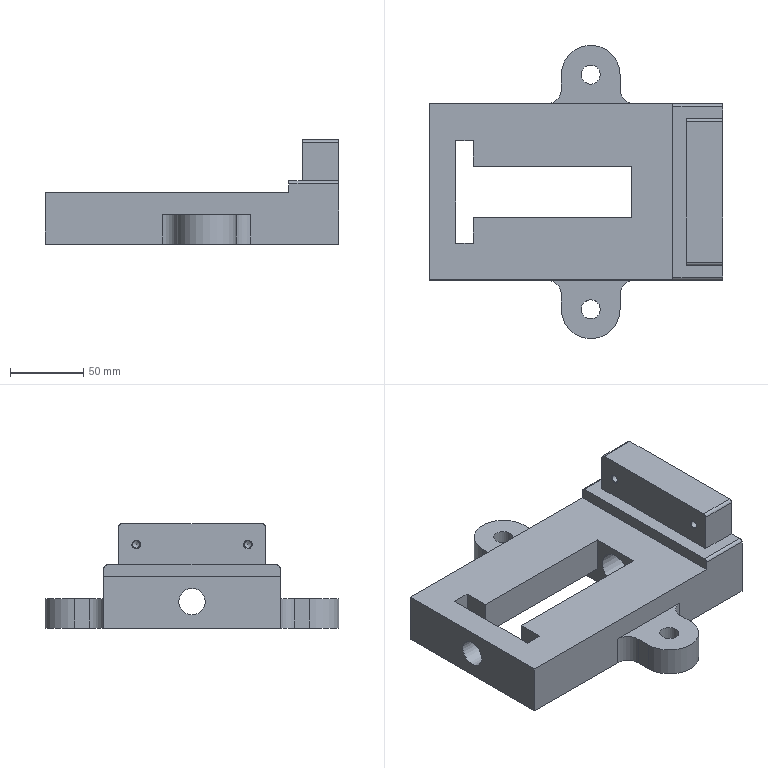Part | NX | features DATUM_CSYS 8, EXTRUDE 7, SKETCH 7, SIMPLE HOLE 4, BLEND 3, HOLE PACKAGE 3, EXTRACT_DATUM_AXIS 2, EXTRACT_DATUM_PLANE 2, EXTRACT_FACE 2, EXTRACT_STRING 2, SYMBOLIC_THREAD 2, BLOCK 1, Instance Feature 1, Mirror Feature 1 | 1 solid | 48 faces | box 200 x 200 x 71 mm | volume 757054 mm3 | plane 28 | cylinder 16 | cone 4 | commonest cylinder face diameters 4 x4 20 x4 5 x2 13 x2 40 x2 18 x1
STEP:
#1=CARTESIAN_POINT('',(-170.,17.5,11.));
#2=VERTEX_POINT('',#1);
#3=CARTESIAN_POINT('',(-62.,17.5,11.));
#4=VERTEX_POINT('',#3);
#5=CARTESIAN_POINT('',(-182.,17.5,11.));
#6=DIRECTION('',(-1.,0.,0.));
#7=VECTOR('',#6,1000.);
#8=LINE('',#5,#7);
#9=EDGE_CURVE('',#2,#4,#8,.F.);
#10=ORIENTED_EDGE('',*,*,#9,.F.);
#11=CARTESIAN_POINT('',(-170.,35.,11.));
#12=VERTEX_POINT('',#11);
#13=CARTESIAN_POINT('',(-170.,0.,11.));
#14=DIRECTION('',(0.,1.,0.));
#15=VECTOR('',#14,1000.);
#16=LINE('',#13,#15);
#17=EDGE_CURVE('',#12,#2,#16,.F.);
#18=ORIENTED_EDGE('',*,*,#17,.F.);
#19=CARTESIAN_POINT('',(-62.,35.,11.));
#20=VERTEX_POINT('',#19);
#21=CARTESIAN_POINT('',(-182.,35.,11.));
#22=DIRECTION('',(1.,0.,0.));
#23=VECTOR('',#22,1000.);
#24=LINE('',#21,#23);
#25=EDGE_CURVE('',#20,#12,#24,.F.);
#26=ORIENTED_EDGE('',*,*,#25,.F.);
#27=CARTESIAN_POINT('',(-62.,0.,11.));
#28=DIRECTION('',(0.,-1.,0.));
#29=VECTOR('',#28,1000.);
#30=LINE('',#27,#29);
#31=EDGE_CURVE('',#4,#20,#30,.F.);
#32=ORIENTED_EDGE('',*,*,#31,.F.);
#33=EDGE_LOOP('',(#10,#18,#26,#32));
#34=FACE_BOUND('',#33,.T.);
#35=CARTESIAN_POINT('',(-182.,0.,11.));
#36=DIRECTION('',(0.,0.,-1.));
#37=DIRECTION('',(1.,0.,0.));
#38=AXIS2_PLACEMENT_3D('',#35,#36,#37);
#39=PLANE('',#38);
#40=ADVANCED_FACE('',(#34),#39,.T.);
#41=ORIENTED_EDGE('',*,*,#17,.T.);
#42=CARTESIAN_POINT('',(-170.,17.5,35.));
#43=VERTEX_POINT('',#42);
#44=CARTESIAN_POINT('',(-170.,17.5,0.));
#45=DIRECTION('',(0.,0.,1.));
#46=VECTOR('',#45,1000.);
#47=LINE('',#44,#46);
#48=EDGE_CURVE('',#2,#43,#47,.T.);
#49=ORIENTED_EDGE('',*,*,#48,.T.);
#50=CARTESIAN_POINT('',(-170.,35.,35.));
#51=VERTEX_POINT('',#50);
#52=CARTESIAN_POINT('',(-170.,0.,35.));
#53=DIRECTION('',(0.,-1.,0.));
#54=VECTOR('',#53,1000.);
#55=LINE('',#52,#54);
#56=EDGE_CURVE('',#43,#51,#55,.F.);
#57=ORIENTED_EDGE('',*,*,#56,.T.);
#58=CARTESIAN_POINT('',(-170.,35.,0.));
#59=DIRECTION('',(0.,0.,1.));
#60=VECTOR('',#59,1000.);
#61=LINE('',#58,#60);
#62=EDGE_CURVE('',#51,#12,#61,.F.);
#63=ORIENTED_EDGE('',*,*,#62,.T.);
#64=EDGE_LOOP('',(#41,#49,#57,#63));
#65=FACE_BOUND('',#64,.T.);
#66=CARTESIAN_POINT('',(-170.,35.,0.));
#67=DIRECTION('',(-1.,0.,0.));
#68=DIRECTION('',(0.,0.,1.));
#69=AXIS2_PLACEMENT_3D('',#66,#67,#68);
#70=PLANE('',#69);
#71=ADVANCED_FACE('',(#65),#70,.T.);
#72=CARTESIAN_POINT('',(-170.,-17.5,35.));
#73=VERTEX_POINT('',#72);
#74=CARTESIAN_POINT('',(-62.,-17.5,35.));
#75=VERTEX_POINT('',#74);
#76=CARTESIAN_POINT('',(-100.,-17.5,35.));
#77=DIRECTION('',(1.,0.,0.));
#78=VECTOR('',#77,1000.);
#79=LINE('',#76,#78);
#80=EDGE_CURVE('',#73,#75,#79,.T.);
#81=ORIENTED_EDGE('',*,*,#80,.F.);
#82=CARTESIAN_POINT('',(-170.,-35.,35.));
#83=VERTEX_POINT('',#82);
#84=CARTESIAN_POINT('',(-170.,0.,35.));
#85=DIRECTION('',(0.,-1.,0.));
#86=VECTOR('',#85,1000.);
#87=LINE('',#84,#86);
#88=EDGE_CURVE('',#83,#73,#87,.F.);
#89=ORIENTED_EDGE('',*,*,#88,.F.);
#90=CARTESIAN_POINT('',(-182.,-35.,35.));
#91=VERTEX_POINT('',#90);
#92=CARTESIAN_POINT('',(-100.,-35.,35.));
#93=DIRECTION('',(1.,0.,0.));
#94=VECTOR('',#93,1000.);
#95=LINE('',#92,#94);
#96=EDGE_CURVE('',#91,#83,#95,.T.);
#97=ORIENTED_EDGE('',*,*,#96,.F.);
#98=CARTESIAN_POINT('',(-182.,35.,35.));
#99=VERTEX_POINT('',#98);
#100=CARTESIAN_POINT('',(-182.,0.,35.));
#101=DIRECTION('',(0.,-1.,0.));
#102=VECTOR('',#101,1000.);
#103=LINE('',#100,#102);
#104=EDGE_CURVE('',#99,#91,#103,.T.);
#105=ORIENTED_EDGE('',*,*,#104,.F.);
#106=CARTESIAN_POINT('',(-100.,35.,35.));
#107=DIRECTION('',(1.,0.,0.));
#108=VECTOR('',#107,1000.);
#109=LINE('',#106,#108);
#110=EDGE_CURVE('',#51,#99,#109,.F.);
#111=ORIENTED_EDGE('',*,*,#110,.F.);
#112=ORIENTED_EDGE('',*,*,#56,.F.);
#113=CARTESIAN_POINT('',(-62.,17.5,35.));
#114=VERTEX_POINT('',#113);
#115=CARTESIAN_POINT('',(-100.,17.5,35.));
#116=DIRECTION('',(1.,0.,0.));
#117=VECTOR('',#116,1000.);
#118=LINE('',#115,#117);
#119=EDGE_CURVE('',#43,#114,#118,.T.);
#120=ORIENTED_EDGE('',*,*,#119,.T.);
#121=CARTESIAN_POINT('',(-62.,0.,35.));
#122=DIRECTION('',(0.,1.,0.));
#123=VECTOR('',#122,1000.);
#124=LINE('',#121,#123);
#125=EDGE_CURVE('',#75,#114,#124,.T.);
#126=ORIENTED_EDGE('',*,*,#125,.F.);
#127=EDGE_LOOP('',(#81,#89,#97,#105,#111,#112,#120,#126));
#128=FACE_BOUND('',#127,.T.);
#129=CARTESIAN_POINT('',(-34.,-60.,35.));
#130=VERTEX_POINT('',#129);
#131=CARTESIAN_POINT('',(-200.,-60.,35.));
#132=VERTEX_POINT('',#131);
#133=CARTESIAN_POINT('',(-100.,-60.,35.));
#134=DIRECTION('',(-1.,0.,0.));
#135=VECTOR('',#134,1000.);
#136=LINE('',#133,#135);
#137=EDGE_CURVE('',#130,#132,#136,.T.);
#138=ORIENTED_EDGE('',*,*,#137,.F.);
#139=CARTESIAN_POINT('',(-34.,60.,35.));
#140=VERTEX_POINT('',#139);
#141=CARTESIAN_POINT('',(-34.,0.,35.));
#142=DIRECTION('',(0.,1.,0.));
#143=VECTOR('',#142,1000.);
#144=LINE('',#141,#143);
#145=EDGE_CURVE('',#130,#140,#144,.T.);
#146=ORIENTED_EDGE('',*,*,#145,.T.);
#147=CARTESIAN_POINT('',(-200.,60.,35.));
#148=VERTEX_POINT('',#147);
#149=CARTESIAN_POINT('',(-100.,60.,35.));
#150=DIRECTION('',(1.,0.,0.));
#151=VECTOR('',#150,1000.);
#152=LINE('',#149,#151);
#153=EDGE_CURVE('',#148,#140,#152,.T.);
#154=ORIENTED_EDGE('',*,*,#153,.F.);
#155=CARTESIAN_POINT('',(-200.,0.,35.));
#156=DIRECTION('',(0.,1.,0.));
#157=VECTOR('',#156,1000.);
#158=LINE('',#155,#157);
#159=EDGE_CURVE('',#132,#148,#158,.T.);
#160=ORIENTED_EDGE('',*,*,#159,.F.);
#161=EDGE_LOOP('',(#138,#146,#154,#160));
#162=FACE_BOUND('',#161,.T.);
#163=CARTESIAN_POINT('',(-100.,0.,35.));
#164=DIRECTION('',(0.,0.,1.));
#165=DIRECTION('',(1.,0.,0.));
#166=AXIS2_PLACEMENT_3D('',#163,#164,#165);
#167=PLANE('',#166);
#168=ADVANCED_FACE('',(#128,#162),#167,.T.);
#169=CARTESIAN_POINT('',(-170.,-17.5,11.));
#170=VERTEX_POINT('',#169);
#171=CARTESIAN_POINT('',(-170.,-35.,11.));
#172=VERTEX_POINT('',#171);
#173=CARTESIAN_POINT('',(-170.,0.,11.));
#174=DIRECTION('',(0.,1.,0.));
#175=VECTOR('',#174,1000.);
#176=LINE('',#173,#175);
#177=EDGE_CURVE('',#170,#172,#176,.F.);
#178=ORIENTED_EDGE('',*,*,#177,.F.);
#179=CARTESIAN_POINT('',(-62.,-17.5,11.));
#180=VERTEX_POINT('',#179);
#181=CARTESIAN_POINT('',(-182.,-17.5,11.));
#182=DIRECTION('',(-1.,0.,0.));
#183=VECTOR('',#182,1000.);
#184=LINE('',#181,#183);
#185=EDGE_CURVE('',#170,#180,#184,.F.);
#186=ORIENTED_EDGE('',*,*,#185,.T.);
#187=CARTESIAN_POINT('',(-62.,-35.,11.));
#188=VERTEX_POINT('',#187);
#189=CARTESIAN_POINT('',(-62.,0.,11.));
#190=DIRECTION('',(0.,-1.,0.));
#191=VECTOR('',#190,1000.);
#192=LINE('',#189,#191);
#193=EDGE_CURVE('',#188,#180,#192,.F.);
#194=ORIENTED_EDGE('',*,*,#193,.F.);
#195=CARTESIAN_POINT('',(-182.,-35.,11.));
#196=DIRECTION('',(1.,0.,0.));
#197=VECTOR('',#196,1000.);
#198=LINE('',#195,#197);
#199=EDGE_CURVE('',#188,#172,#198,.F.);
#200=ORIENTED_EDGE('',*,*,#199,.T.);
#201=EDGE_LOOP('',(#178,#186,#194,#200));
#202=FACE_BOUND('',#201,.T.);
#203=CARTESIAN_POINT('',(-182.,0.,11.));
#204=DIRECTION('',(0.,0.,-1.));
#205=DIRECTION('',(1.,0.,0.));
#206=AXIS2_PLACEMENT_3D('',#203,#204,#205);
#207=PLANE('',#206);
#208=ADVANCED_FACE('',(#202),#207,.T.);
#209=CARTESIAN_POINT('',(0.,60.,0.));
#210=VERTEX_POINT('',#209);
#211=CARTESIAN_POINT('',(-60.,60.,0.));
#212=VERTEX_POINT('',#211);
#213=CARTESIAN_POINT('',(-100.,60.,0.));
#214=DIRECTION('',(-1.,0.,0.));
#215=VECTOR('',#214,1000.);
#216=LINE('',#213,#215);
#217=EDGE_CURVE('',#210,#212,#216,.T.);
#218=ORIENTED_EDGE('',*,*,#217,.F.);
#219=CARTESIAN_POINT('',(0.,-60.,0.));
#220=VERTEX_POINT('',#219);
#221=CARTESIAN_POINT('',(0.,0.,0.));
#222=DIRECTION('',(0.,1.,0.));
#223=VECTOR('',#222,1000.);
#224=LINE('',#221,#223);
#225=EDGE_CURVE('',#220,#210,#224,.T.);
#226=ORIENTED_EDGE('',*,*,#225,.F.);
#227=CARTESIAN_POINT('',(-60.,-60.,0.));
#228=VERTEX_POINT('',#227);
#229=CARTESIAN_POINT('',(-100.,-60.,0.));
#230=DIRECTION('',(1.,0.,0.));
#231=VECTOR('',#230,1000.);
#232=LINE('',#229,#231);
#233=EDGE_CURVE('',#228,#220,#232,.T.);
#234=ORIENTED_EDGE('',*,*,#233,.F.);
#235=CARTESIAN_POINT('',(-70.,-70.,0.));
#236=VERTEX_POINT('',#235);
#237=CARTESIAN_POINT('',(-60.,-70.,0.));
#238=DIRECTION('',(0.,0.,-1.));
#239=DIRECTION('',(-1.,0.,0.));
#240=AXIS2_PLACEMENT_3D('',#237,#238,#239);
#241=CIRCLE('',#240,10.);
#242=EDGE_CURVE('',#228,#236,#241,.F.);
#243=ORIENTED_EDGE('',*,*,#242,.T.);
#244=CARTESIAN_POINT('',(-70.,-80.,0.));
#245=VERTEX_POINT('',#244);
#246=CARTESIAN_POINT('',(-70.,-80.,0.));
#247=DIRECTION('',(0.,1.,0.));
#248=VECTOR('',#247,1000.);
#249=LINE('',#246,#248);
#250=EDGE_CURVE('',#245,#236,#249,.T.);
#251=ORIENTED_EDGE('',*,*,#250,.F.);
#252=CARTESIAN_POINT('',(-110.,-80.,0.));
#253=VERTEX_POINT('',#252);
#254=CARTESIAN_POINT('',(-90.,-80.,0.));
#255=DIRECTION('',(0.,0.,1.));
#256=DIRECTION('',(1.,0.,0.));
#257=AXIS2_PLACEMENT_3D('',#254,#255,#256);
#258=CIRCLE('',#257,20.);
#259=EDGE_CURVE('',#253,#245,#258,.T.);
#260=ORIENTED_EDGE('',*,*,#259,.F.);
#261=CARTESIAN_POINT('',(-110.,-70.,0.));
#262=VERTEX_POINT('',#261);
#263=CARTESIAN_POINT('',(-110.,-60.,0.));
#264=DIRECTION('',(0.,-1.,0.));
#265=VECTOR('',#264,1000.);
#266=LINE('',#263,#265);
#267=EDGE_CURVE('',#262,#253,#266,.T.);
#268=ORIENTED_EDGE('',*,*,#267,.F.);
#269=CARTESIAN_POINT('',(-120.,-60.,0.));
#270=VERTEX_POINT('',#269);
#271=CARTESIAN_POINT('',(-120.,-70.,0.));
#272=DIRECTION('',(0.,0.,-1.));
#273=DIRECTION('',(-1.,0.,0.));
#274=AXIS2_PLACEMENT_3D('',#271,#272,#273);
#275=CIRCLE('',#274,10.);
#276=EDGE_CURVE('',#262,#270,#275,.F.);
#277=ORIENTED_EDGE('',*,*,#276,.T.);
#278=CARTESIAN_POINT('',(-200.,-60.,0.));
#279=VERTEX_POINT('',#278);
#280=CARTESIAN_POINT('',(-100.,-60.,0.));
#281=DIRECTION('',(1.,0.,0.));
#282=VECTOR('',#281,1000.);
#283=LINE('',#280,#282);
#284=EDGE_CURVE('',#279,#270,#283,.T.);
#285=ORIENTED_EDGE('',*,*,#284,.F.);
#286=CARTESIAN_POINT('',(-200.,60.,0.));
#287=VERTEX_POINT('',#286);
#288=CARTESIAN_POINT('',(-200.,0.,0.));
#289=DIRECTION('',(0.,-1.,0.));
#290=VECTOR('',#289,1000.);
#291=LINE('',#288,#290);
#292=EDGE_CURVE('',#287,#279,#291,.T.);
#293=ORIENTED_EDGE('',*,*,#292,.F.);
#294=CARTESIAN_POINT('',(-120.,60.,0.));
#295=VERTEX_POINT('',#294);
#296=CARTESIAN_POINT('',(-100.,60.,0.));
#297=DIRECTION('',(-1.,0.,0.));
#298=VECTOR('',#297,1000.);
#299=LINE('',#296,#298);
#300=EDGE_CURVE('',#295,#287,#299,.T.);
#301=ORIENTED_EDGE('',*,*,#300,.F.);
#302=CARTESIAN_POINT('',(-110.,70.,0.));
#303=VERTEX_POINT('',#302);
#304=CARTESIAN_POINT('',(-120.,70.,0.));
#305=DIRECTION('',(0.,0.,-1.));
#306=DIRECTION('',(-1.,0.,0.));
#307=AXIS2_PLACEMENT_3D('',#304,#305,#306);
#308=CIRCLE('',#307,10.);
#309=EDGE_CURVE('',#295,#303,#308,.F.);
#310=ORIENTED_EDGE('',*,*,#309,.T.);
#311=CARTESIAN_POINT('',(-110.,80.,0.));
#312=VERTEX_POINT('',#311);
#313=CARTESIAN_POINT('',(-110.,60.,0.));
#314=DIRECTION('',(0.,1.,0.));
#315=VECTOR('',#314,1000.);
#316=LINE('',#313,#315);
#317=EDGE_CURVE('',#303,#312,#316,.T.);
#318=ORIENTED_EDGE('',*,*,#317,.T.);
#319=CARTESIAN_POINT('',(-70.,80.,0.));
#320=VERTEX_POINT('',#319);
#321=CARTESIAN_POINT('',(-90.,80.,0.));
#322=DIRECTION('',(0.,0.,-1.));
#323=DIRECTION('',(1.,0.,0.));
#324=AXIS2_PLACEMENT_3D('',#321,#322,#323);
#325=CIRCLE('',#324,20.);
#326=EDGE_CURVE('',#312,#320,#325,.T.);
#327=ORIENTED_EDGE('',*,*,#326,.T.);
#328=CARTESIAN_POINT('',(-70.,70.,0.));
#329=VERTEX_POINT('',#328);
#330=CARTESIAN_POINT('',(-70.,80.,0.));
#331=DIRECTION('',(0.,-1.,0.));
#332=VECTOR('',#331,1000.);
#333=LINE('',#330,#332);
#334=EDGE_CURVE('',#320,#329,#333,.T.);
#335=ORIENTED_EDGE('',*,*,#334,.T.);
#336=CARTESIAN_POINT('',(-60.,70.,0.));
#337=DIRECTION('',(0.,0.,-1.));
#338=DIRECTION('',(-1.,0.,0.));
#339=AXIS2_PLACEMENT_3D('',#336,#337,#338);
#340=CIRCLE('',#339,10.);
#341=EDGE_CURVE('',#329,#212,#340,.F.);
#342=ORIENTED_EDGE('',*,*,#341,.T.);
#343=EDGE_LOOP('',(#218,#226,#234,#243,#251,#260,#268,#277,#285,#293,#301,#310,#318,#327,#335,#342));
#344=FACE_BOUND('',#343,.T.);
#345=CARTESIAN_POINT('',(-182.,35.,0.));
#346=VERTEX_POINT('',#345);
#347=CARTESIAN_POINT('',(-182.,-35.,0.));
#348=VERTEX_POINT('',#347);
#349=CARTESIAN_POINT('',(-182.,0.,0.));
#350=DIRECTION('',(0.,-1.,0.));
#351=VECTOR('',#350,1000.);
#352=LINE('',#349,#351);
#353=EDGE_CURVE('',#346,#348,#352,.T.);
#354=ORIENTED_EDGE('',*,*,#353,.T.);
#355=CARTESIAN_POINT('',(-62.,-35.,0.));
#356=VERTEX_POINT('',#355);
#357=CARTESIAN_POINT('',(-182.,-35.,0.));
#358=DIRECTION('',(1.,0.,0.));
#359=VECTOR('',#358,1000.);
#360=LINE('',#357,#359);
#361=EDGE_CURVE('',#348,#356,#360,.T.);
#362=ORIENTED_EDGE('',*,*,#361,.T.);
#363=CARTESIAN_POINT('',(-62.,35.,0.));
#364=VERTEX_POINT('',#363);
#365=CARTESIAN_POINT('',(-62.,0.,0.));
#366=DIRECTION('',(0.,-1.,0.));
#367=VECTOR('',#366,1000.);
#368=LINE('',#365,#367);
#369=EDGE_CURVE('',#364,#356,#368,.T.);
#370=ORIENTED_EDGE('',*,*,#369,.F.);
#371=CARTESIAN_POINT('',(-182.,35.,0.));
#372=DIRECTION('',(1.,0.,0.));
#373=VECTOR('',#372,1000.);
#374=LINE('',#371,#373);
#375=EDGE_CURVE('',#346,#364,#374,.T.);
#376=ORIENTED_EDGE('',*,*,#375,.F.);
#377=EDGE_LOOP('',(#354,#362,#370,#376));
#378=FACE_BOUND('',#377,.T.);
#379=CARTESIAN_POINT('',(-83.5,-80.,0.));
#380=VERTEX_POINT('',#379);
#381=CARTESIAN_POINT('',(-90.,-80.,0.));
#382=DIRECTION('',(0.,0.,1.));
#383=DIRECTION('',(1.,0.,0.));
#384=AXIS2_PLACEMENT_3D('',#381,#382,#383);
#385=CIRCLE('',#384,6.5);
#386=EDGE_CURVE('',#380,#380,#385,.T.);
#387=ORIENTED_EDGE('',*,*,#386,.T.);
#388=EDGE_LOOP('',(#387));
#389=FACE_BOUND('',#388,.T.);
#390=CARTESIAN_POINT('',(-83.5,80.,0.));
#391=VERTEX_POINT('',#390);
#392=CARTESIAN_POINT('',(-90.,80.,0.));
#393=DIRECTION('',(0.,0.,-1.));
#394=DIRECTION('',(1.,0.,0.));
#395=AXIS2_PLACEMENT_3D('',#392,#393,#394);
#396=CIRCLE('',#395,6.5);
#397=EDGE_CURVE('',#391,#391,#396,.T.);
#398=ORIENTED_EDGE('',*,*,#397,.F.);
#399=EDGE_LOOP('',(#398));
#400=FACE_BOUND('',#399,.T.);
#401=CARTESIAN_POINT('',(-100.,0.,0.));
#402=DIRECTION('',(0.,0.,-1.));
#403=DIRECTION('',(-1.,0.,0.));
#404=AXIS2_PLACEMENT_3D('',#401,#402,#403);
#405=PLANE('',#404);
#406=ADVANCED_FACE('',(#344,#378,#389,#400),#405,.T.);
#407=CARTESIAN_POINT('',(0.,-60.,41.));
#408=VERTEX_POINT('',#407);
#409=CARTESIAN_POINT('',(0.,-60.,0.));
#410=DIRECTION('',(0.,0.,1.));
#411=VECTOR('',#410,1000.);
#412=LINE('',#409,#411);
#413=EDGE_CURVE('',#220,#408,#412,.T.);
#414=ORIENTED_EDGE('',*,*,#413,.T.);
#415=CARTESIAN_POINT('',(-34.,-60.,41.));
#416=VERTEX_POINT('',#415);
#417=CARTESIAN_POINT('',(-34.,-60.,41.));
#418=DIRECTION('',(-1.,0.,0.));
#419=VECTOR('',#418,1000.);
#420=LINE('',#417,#419);
#421=EDGE_CURVE('',#408,#416,#420,.T.);
#422=ORIENTED_EDGE('',*,*,#421,.T.);
#423=CARTESIAN_POINT('',(-34.,-60.,0.));
#424=DIRECTION('',(0.,0.,-1.));
#425=VECTOR('',#424,1000.);
#426=LINE('',#423,#425);
#427=EDGE_CURVE('',#130,#416,#426,.F.);
#428=ORIENTED_EDGE('',*,*,#427,.F.);
#429=ORIENTED_EDGE('',*,*,#137,.T.);
#430=CARTESIAN_POINT('',(-200.,-60.,0.));
#431=DIRECTION('',(0.,0.,1.));
#432=VECTOR('',#431,1000.);
#433=LINE('',#430,#432);
#434=EDGE_CURVE('',#279,#132,#433,.T.);
#435=ORIENTED_EDGE('',*,*,#434,.F.);
#436=ORIENTED_EDGE('',*,*,#284,.T.);
#437=CARTESIAN_POINT('',(-120.,-60.,20.));
#438=VERTEX_POINT('',#437);
#439=CARTESIAN_POINT('',(-120.,-60.,0.));
#440=DIRECTION('',(0.,0.,-1.));
#441=VECTOR('',#440,1000.);
#442=LINE('',#439,#441);
#443=EDGE_CURVE('',#270,#438,#442,.F.);
#444=ORIENTED_EDGE('',*,*,#443,.T.);
#445=CARTESIAN_POINT('',(-60.,-60.,20.));
#446=VERTEX_POINT('',#445);
#447=CARTESIAN_POINT('',(-70.,-60.,20.));
#448=DIRECTION('',(-1.,0.,0.));
#449=VECTOR('',#448,1000.);
#450=LINE('',#447,#449);
#451=EDGE_CURVE('',#446,#438,#450,.T.);
#452=ORIENTED_EDGE('',*,*,#451,.F.);
#453=CARTESIAN_POINT('',(-60.,-60.,0.));
#454=DIRECTION('',(0.,0.,-1.));
#455=VECTOR('',#454,1000.);
#456=LINE('',#453,#455);
#457=EDGE_CURVE('',#446,#228,#456,.T.);
#458=ORIENTED_EDGE('',*,*,#457,.T.);
#459=ORIENTED_EDGE('',*,*,#233,.T.);
#460=EDGE_LOOP('',(#414,#422,#428,#429,#435,#436,#444,#452,#458,#459));
#461=FACE_BOUND('',#460,.T.);
#462=CARTESIAN_POINT('',(-100.,-60.,0.));
#463=DIRECTION('',(0.,-1.,0.));
#464=DIRECTION('',(0.,0.,-1.));
#465=AXIS2_PLACEMENT_3D('',#462,#463,#464);
#466=PLANE('',#465);
#467=ADVANCED_FACE('',(#461),#466,.T.);
#468=CARTESIAN_POINT('',(-200.,0.,9.));
#469=VERTEX_POINT('',#468);
#470=CARTESIAN_POINT('',(-200.,0.,18.));
#471=DIRECTION('',(1.,0.,0.));
#472=DIRECTION('',(0.,0.,-1.));
#473=AXIS2_PLACEMENT_3D('',#470,#471,#472);
#474=CIRCLE('',#473,9.);
#475=EDGE_CURVE('',#469,#469,#474,.T.);
#476=ORIENTED_EDGE('',*,*,#475,.T.);
#477=EDGE_LOOP('',(#476));
#478=FACE_BOUND('',#477,.T.);
#479=ORIENTED_EDGE('',*,*,#434,.T.);
#480=ORIENTED_EDGE('',*,*,#159,.T.);
#481=CARTESIAN_POINT('',(-200.,60.,0.));
#482=DIRECTION('',(0.,0.,1.));
#483=VECTOR('',#482,1000.);
#484=LINE('',#481,#483);
#485=EDGE_CURVE('',#287,#148,#484,.T.);
#486=ORIENTED_EDGE('',*,*,#485,.F.);
#487=ORIENTED_EDGE('',*,*,#292,.T.);
#488=EDGE_LOOP('',(#479,#480,#486,#487));
#489=FACE_BOUND('',#488,.T.);
#490=CARTESIAN_POINT('',(-200.,0.,0.));
#491=DIRECTION('',(-1.,0.,0.));
#492=DIRECTION('',(0.,0.,1.));
#493=AXIS2_PLACEMENT_3D('',#490,#491,#492);
#494=PLANE('',#493);
#495=ADVANCED_FACE('',(#478,#489),#494,.T.);
#496=CARTESIAN_POINT('',(-34.,60.,41.));
#497=VERTEX_POINT('',#496);
#498=CARTESIAN_POINT('',(-34.,60.,0.));
#499=DIRECTION('',(0.,0.,-1.));
#500=VECTOR('',#499,1000.);
#501=LINE('',#498,#500);
#502=EDGE_CURVE('',#140,#497,#501,.F.);
#503=ORIENTED_EDGE('',*,*,#502,.T.);
#504=CARTESIAN_POINT('',(0.,60.,41.));
#505=VERTEX_POINT('',#504);
#506=CARTESIAN_POINT('',(0.,60.,41.));
#507=DIRECTION('',(-1.,0.,0.));
#508=VECTOR('',#507,1000.);
#509=LINE('',#506,#508);
#510=EDGE_CURVE('',#497,#505,#509,.F.);
#511=ORIENTED_EDGE('',*,*,#510,.T.);
#512=CARTESIAN_POINT('',(0.,60.,0.));
#513=DIRECTION('',(0.,0.,1.));
#514=VECTOR('',#513,1000.);
#515=LINE('',#512,#514);
#516=EDGE_CURVE('',#210,#505,#515,.T.);
#517=ORIENTED_EDGE('',*,*,#516,.F.);
#518=ORIENTED_EDGE('',*,*,#217,.T.);
#519=CARTESIAN_POINT('',(-60.,60.,20.));
#520=VERTEX_POINT('',#519);
#521=CARTESIAN_POINT('',(-60.,60.,20.));
#522=DIRECTION('',(0.,0.,-1.));
#523=VECTOR('',#522,1000.);
#524=LINE('',#521,#523);
#525=EDGE_CURVE('',#212,#520,#524,.F.);
#526=ORIENTED_EDGE('',*,*,#525,.T.);
#527=CARTESIAN_POINT('',(-120.,60.,20.));
#528=VERTEX_POINT('',#527);
#529=CARTESIAN_POINT('',(-70.,60.,20.));
#530=DIRECTION('',(-1.,0.,0.));
#531=VECTOR('',#530,1000.);
#532=LINE('',#529,#531);
#533=EDGE_CURVE('',#520,#528,#532,.T.);
#534=ORIENTED_EDGE('',*,*,#533,.T.);
#535=CARTESIAN_POINT('',(-120.,60.,0.));
#536=DIRECTION('',(0.,0.,-1.));
#537=VECTOR('',#536,1000.);
#538=LINE('',#535,#537);
#539=EDGE_CURVE('',#528,#295,#538,.T.);
#540=ORIENTED_EDGE('',*,*,#539,.T.);
#541=ORIENTED_EDGE('',*,*,#300,.T.);
#542=ORIENTED_EDGE('',*,*,#485,.T.);
#543=ORIENTED_EDGE('',*,*,#153,.T.);
#544=EDGE_LOOP('',(#503,#511,#517,#518,#526,#534,#540,#541,#542,#543));
#545=FACE_BOUND('',#544,.T.);
#546=CARTESIAN_POINT('',(-100.,60.,0.));
#547=DIRECTION('',(0.,1.,0.));
#548=DIRECTION('',(0.,0.,1.));
#549=AXIS2_PLACEMENT_3D('',#546,#547,#548);
#550=PLANE('',#549);
#551=ADVANCED_FACE('',(#545),#550,.T.);
#552=CARTESIAN_POINT('',(0.,0.,30.5));
#553=VERTEX_POINT('',#552);
#554=CARTESIAN_POINT('',(0.,0.,18.));
#555=DIRECTION('',(-1.,0.,0.));
#556=DIRECTION('',(0.,0.,1.));
#557=AXIS2_PLACEMENT_3D('',#554,#555,#556);
#558=CIRCLE('',#557,12.5);
#559=EDGE_CURVE('',#553,#553,#558,.T.);
#560=ORIENTED_EDGE('',*,*,#559,.T.);
#561=EDGE_LOOP('',(#560));
#562=FACE_BOUND('',#561,.T.);
#563=CARTESIAN_POINT('',(0.,50.,43.));
#564=VERTEX_POINT('',#563);
#565=CARTESIAN_POINT('',(0.,50.,69.));
#566=VERTEX_POINT('',#565);
#567=CARTESIAN_POINT('',(0.,50.,0.));
#568=DIRECTION('',(0.,0.,1.));
#569=VECTOR('',#568,1000.);
#570=LINE('',#567,#569);
#571=EDGE_CURVE('',#564,#566,#570,.T.);
#572=ORIENTED_EDGE('',*,*,#571,.T.);
#573=CARTESIAN_POINT('',(0.,48.,71.));
#574=VERTEX_POINT('',#573);
#575=CARTESIAN_POINT('',(0.,48.,69.));
#576=DIRECTION('',(1.,0.,0.));
#577=DIRECTION('',(0.,0.,-1.));
#578=AXIS2_PLACEMENT_3D('',#575,#576,#577);
#579=CIRCLE('',#578,2.);
#580=EDGE_CURVE('',#566,#574,#579,.T.);
#581=ORIENTED_EDGE('',*,*,#580,.T.);
#582=CARTESIAN_POINT('',(0.,-48.,71.));
#583=VERTEX_POINT('',#582);
#584=CARTESIAN_POINT('',(0.,0.,71.));
#585=DIRECTION('',(0.,1.,0.));
#586=VECTOR('',#585,1000.);
#587=LINE('',#584,#586);
#588=EDGE_CURVE('',#583,#574,#587,.T.);
#589=ORIENTED_EDGE('',*,*,#588,.F.);
#590=CARTESIAN_POINT('',(0.,-50.,69.));
#591=VERTEX_POINT('',#590);
#592=CARTESIAN_POINT('',(0.,-48.,69.));
#593=DIRECTION('',(1.,0.,0.));
#594=DIRECTION('',(0.,0.,-1.));
#595=AXIS2_PLACEMENT_3D('',#592,#593,#594);
#596=CIRCLE('',#595,2.);
#597=EDGE_CURVE('',#583,#591,#596,.T.);
#598=ORIENTED_EDGE('',*,*,#597,.T.);
#599=CARTESIAN_POINT('',(0.,-50.,43.));
#600=VERTEX_POINT('',#599);
#601=CARTESIAN_POINT('',(0.,-50.,0.));
#602=DIRECTION('',(0.,0.,1.));
#603=VECTOR('',#602,1000.);
#604=LINE('',#601,#603);
#605=EDGE_CURVE('',#600,#591,#604,.T.);
#606=ORIENTED_EDGE('',*,*,#605,.F.);
#607=CARTESIAN_POINT('',(0.,-58.,43.));
#608=VERTEX_POINT('',#607);
#609=CARTESIAN_POINT('',(0.,-60.,43.));
#610=DIRECTION('',(0.,1.,0.));
#611=VECTOR('',#610,1000.);
#612=LINE('',#609,#611);
#613=EDGE_CURVE('',#608,#600,#612,.T.);
#614=ORIENTED_EDGE('',*,*,#613,.F.);
#615=CARTESIAN_POINT('',(0.,-58.,41.));
#616=DIRECTION('',(1.,0.,0.));
#617=DIRECTION('',(0.,0.,-1.));
#618=AXIS2_PLACEMENT_3D('',#615,#616,#617);
#619=CIRCLE('',#618,2.);
#620=EDGE_CURVE('',#608,#408,#619,.T.);
#621=ORIENTED_EDGE('',*,*,#620,.T.);
#622=ORIENTED_EDGE('',*,*,#413,.F.);
#623=ORIENTED_EDGE('',*,*,#225,.T.);
#624=ORIENTED_EDGE('',*,*,#516,.T.);
#625=CARTESIAN_POINT('',(0.,58.,43.));
#626=VERTEX_POINT('',#625);
#627=CARTESIAN_POINT('',(0.,58.,41.));
#628=DIRECTION('',(1.,0.,0.));
#629=DIRECTION('',(0.,0.,-1.));
#630=AXIS2_PLACEMENT_3D('',#627,#628,#629);
#631=CIRCLE('',#630,2.);
#632=EDGE_CURVE('',#505,#626,#631,.T.);
#633=ORIENTED_EDGE('',*,*,#632,.T.);
#634=CARTESIAN_POINT('',(0.,-60.,43.));
#635=DIRECTION('',(0.,1.,0.));
#636=VECTOR('',#635,1000.);
#637=LINE('',#634,#636);
#638=EDGE_CURVE('',#564,#626,#637,.T.);
#639=ORIENTED_EDGE('',*,*,#638,.F.);
#640=EDGE_LOOP('',(#572,#581,#589,#598,#606,#614,#621,#622,#623,#624,#633,#639));
#641=FACE_BOUND('',#640,.T.);
#642=CARTESIAN_POINT('',(0.,0.,0.));
#643=DIRECTION('',(1.,0.,0.));
#644=DIRECTION('',(0.,0.,-1.));
#645=AXIS2_PLACEMENT_3D('',#642,#643,#644);
#646=PLANE('',#645);
#647=ADVANCED_FACE('',(#562,#641),#646,.T.);
#648=ORIENTED_EDGE('',*,*,#638,.T.);
#649=CARTESIAN_POINT('',(-34.,58.,43.));
#650=VERTEX_POINT('',#649);
#651=CARTESIAN_POINT('',(-34.,58.,43.));
#652=DIRECTION('',(-1.,0.,0.));
#653=VECTOR('',#652,1000.);
#654=LINE('',#651,#653);
#655=EDGE_CURVE('',#626,#650,#654,.T.);
#656=ORIENTED_EDGE('',*,*,#655,.T.);
#657=CARTESIAN_POINT('',(-34.,-58.,43.));
#658=VERTEX_POINT('',#657);
#659=CARTESIAN_POINT('',(-34.,-60.,43.));
#660=DIRECTION('',(0.,1.,0.));
#661=VECTOR('',#660,1000.);
#662=LINE('',#659,#661);
#663=EDGE_CURVE('',#658,#650,#662,.T.);
#664=ORIENTED_EDGE('',*,*,#663,.F.);
#665=CARTESIAN_POINT('',(0.,-58.,43.));
#666=DIRECTION('',(-1.,0.,0.));
#667=VECTOR('',#666,1000.);
#668=LINE('',#665,#667);
#669=EDGE_CURVE('',#658,#608,#668,.F.);
#670=ORIENTED_EDGE('',*,*,#669,.T.);
#671=ORIENTED_EDGE('',*,*,#613,.T.);
#672=CARTESIAN_POINT('',(-25.,-50.,43.));
#673=VERTEX_POINT('',#672);
#674=CARTESIAN_POINT('',(0.,-50.,43.));
#675=DIRECTION('',(1.,0.,0.));
#676=VECTOR('',#675,1000.);
#677=LINE('',#674,#676);
#678=EDGE_CURVE('',#673,#600,#677,.T.);
#679=ORIENTED_EDGE('',*,*,#678,.F.);
#680=CARTESIAN_POINT('',(-25.,50.,43.));
#681=VERTEX_POINT('',#680);
#682=CARTESIAN_POINT('',(-25.,-60.,43.));
#683=DIRECTION('',(0.,1.,0.));
#684=VECTOR('',#683,1000.);
#685=LINE('',#682,#684);
#686=EDGE_CURVE('',#673,#681,#685,.T.);
#687=ORIENTED_EDGE('',*,*,#686,.T.);
#688=CARTESIAN_POINT('',(0.,50.,43.));
#689=DIRECTION('',(1.,0.,0.));
#690=VECTOR('',#689,1000.);
#691=LINE('',#688,#690);
#692=EDGE_CURVE('',#681,#564,#691,.T.);
#693=ORIENTED_EDGE('',*,*,#692,.T.);
#694=EDGE_LOOP('',(#648,#656,#664,#670,#671,#679,#687,#693));
#695=FACE_BOUND('',#694,.T.);
#696=CARTESIAN_POINT('',(0.,-60.,43.));
#697=DIRECTION('',(0.,0.,-1.));
#698=DIRECTION('',(0.,1.,0.));
#699=AXIS2_PLACEMENT_3D('',#696,#697,#698);
#700=PLANE('',#699);
#701=ADVANCED_FACE('',(#695),#700,.F.);
#702=ORIENTED_EDGE('',*,*,#663,.T.);
#703=CARTESIAN_POINT('',(-34.,58.,41.));
#704=DIRECTION('',(1.,0.,0.));
#705=DIRECTION('',(0.,0.,-1.));
#706=AXIS2_PLACEMENT_3D('',#703,#704,#705);
#707=CIRCLE('',#706,2.);
#708=EDGE_CURVE('',#650,#497,#707,.F.);
#709=ORIENTED_EDGE('',*,*,#708,.T.);
#710=ORIENTED_EDGE('',*,*,#502,.F.);
#711=ORIENTED_EDGE('',*,*,#145,.F.);
#712=ORIENTED_EDGE('',*,*,#427,.T.);
#713=CARTESIAN_POINT('',(-34.,-58.,41.));
#714=DIRECTION('',(1.,0.,0.));
#715=DIRECTION('',(0.,0.,-1.));
#716=AXIS2_PLACEMENT_3D('',#713,#714,#715);
#717=CIRCLE('',#716,2.);
#718=EDGE_CURVE('',#416,#658,#717,.F.);
#719=ORIENTED_EDGE('',*,*,#718,.T.);
#720=EDGE_LOOP('',(#702,#709,#710,#711,#712,#719));
#721=FACE_BOUND('',#720,.T.);
#722=CARTESIAN_POINT('',(-34.,-60.,0.));
#723=DIRECTION('',(1.,0.,0.));
#724=DIRECTION('',(0.,0.,-1.));
#725=AXIS2_PLACEMENT_3D('',#722,#723,#724);
#726=PLANE('',#725);
#727=ADVANCED_FACE('',(#721),#726,.F.);
#728=CARTESIAN_POINT('',(-25.,35.,57.));
#729=VERTEX_POINT('',#728);
#730=CARTESIAN_POINT('',(-25.,38.,57.));
#731=DIRECTION('',(-1.,0.,0.));
#732=DIRECTION('',(0.,-1.,0.));
#733=AXIS2_PLACEMENT_3D('',#730,#731,#732);
#734=CIRCLE('',#733,3.);
#735=EDGE_CURVE('',#729,#729,#734,.F.);
#736=ORIENTED_EDGE('',*,*,#735,.T.);
#737=EDGE_LOOP('',(#736));
#738=FACE_BOUND('',#737,.T.);
#739=CARTESIAN_POINT('',(-25.,-41.,57.));
#740=VERTEX_POINT('',#739);
#741=CARTESIAN_POINT('',(-25.,-38.,57.));
#742=DIRECTION('',(-1.,0.,0.));
#743=DIRECTION('',(0.,-1.,0.));
#744=AXIS2_PLACEMENT_3D('',#741,#742,#743);
#745=CIRCLE('',#744,3.);
#746=EDGE_CURVE('',#740,#740,#745,.F.);
#747=ORIENTED_EDGE('',*,*,#746,.T.);
#748=EDGE_LOOP('',(#747));
#749=FACE_BOUND('',#748,.T.);
#750=CARTESIAN_POINT('',(-25.,-48.,71.));
#751=VERTEX_POINT('',#750);
#752=CARTESIAN_POINT('',(-25.,48.,71.));
#753=VERTEX_POINT('',#752);
#754=CARTESIAN_POINT('',(-25.,0.,71.));
#755=DIRECTION('',(0.,1.,0.));
#756=VECTOR('',#755,1000.);
#757=LINE('',#754,#756);
#758=EDGE_CURVE('',#751,#753,#757,.T.);
#759=ORIENTED_EDGE('',*,*,#758,.T.);
#760=CARTESIAN_POINT('',(-25.,50.,69.));
#761=VERTEX_POINT('',#760);
#762=CARTESIAN_POINT('',(-25.,48.,69.));
#763=DIRECTION('',(-1.,0.,0.));
#764=DIRECTION('',(0.,-1.,0.));
#765=AXIS2_PLACEMENT_3D('',#762,#763,#764);
#766=CIRCLE('',#765,2.);
#767=EDGE_CURVE('',#753,#761,#766,.T.);
#768=ORIENTED_EDGE('',*,*,#767,.T.);
#769=CARTESIAN_POINT('',(-25.,50.,0.));
#770=DIRECTION('',(0.,0.,1.));
#771=VECTOR('',#770,1000.);
#772=LINE('',#769,#771);
#773=EDGE_CURVE('',#681,#761,#772,.T.);
#774=ORIENTED_EDGE('',*,*,#773,.F.);
#775=ORIENTED_EDGE('',*,*,#686,.F.);
#776=CARTESIAN_POINT('',(-25.,-50.,69.));
#777=VERTEX_POINT('',#776);
#778=CARTESIAN_POINT('',(-25.,-50.,0.));
#779=DIRECTION('',(0.,0.,1.));
#780=VECTOR('',#779,1000.);
#781=LINE('',#778,#780);
#782=EDGE_CURVE('',#673,#777,#781,.T.);
#783=ORIENTED_EDGE('',*,*,#782,.T.);
#784=CARTESIAN_POINT('',(-25.,-48.,69.));
#785=DIRECTION('',(-1.,0.,0.));
#786=DIRECTION('',(0.,-1.,0.));
#787=AXIS2_PLACEMENT_3D('',#784,#785,#786);
#788=CIRCLE('',#787,2.);
#789=EDGE_CURVE('',#777,#751,#788,.T.);
#790=ORIENTED_EDGE('',*,*,#789,.T.);
#791=EDGE_LOOP('',(#759,#768,#774,#775,#783,#790));
#792=FACE_BOUND('',#791,.T.);
#793=CARTESIAN_POINT('',(-25.,0.,0.));
#794=DIRECTION('',(-1.,0.,0.));
#795=DIRECTION('',(0.,0.,1.));
#796=AXIS2_PLACEMENT_3D('',#793,#794,#795);
#797=PLANE('',#796);
#798=ADVANCED_FACE('',(#738,#749,#792),#797,.T.);
#799=ORIENTED_EDGE('',*,*,#773,.T.);
#800=CARTESIAN_POINT('',(0.,50.,69.));
#801=DIRECTION('',(1.,0.,0.));
#802=VECTOR('',#801,1000.);
#803=LINE('',#800,#802);
#804=EDGE_CURVE('',#761,#566,#803,.T.);
#805=ORIENTED_EDGE('',*,*,#804,.T.);
#806=ORIENTED_EDGE('',*,*,#571,.F.);
#807=ORIENTED_EDGE('',*,*,#692,.F.);
#808=EDGE_LOOP('',(#799,#805,#806,#807));
#809=FACE_BOUND('',#808,.T.);
#810=CARTESIAN_POINT('',(0.,50.,0.));
#811=DIRECTION('',(0.,1.,0.));
#812=DIRECTION('',(-1.,0.,0.));
#813=AXIS2_PLACEMENT_3D('',#810,#811,#812);
#814=PLANE('',#813);
#815=ADVANCED_FACE('',(#809),#814,.T.);
#816=ORIENTED_EDGE('',*,*,#605,.T.);
#817=CARTESIAN_POINT('',(-25.,-50.,69.));
#818=DIRECTION('',(1.,0.,0.));
#819=VECTOR('',#818,1000.);
#820=LINE('',#817,#819);
#821=EDGE_CURVE('',#591,#777,#820,.F.);
#822=ORIENTED_EDGE('',*,*,#821,.T.);
#823=ORIENTED_EDGE('',*,*,#782,.F.);
#824=ORIENTED_EDGE('',*,*,#678,.T.);
#825=EDGE_LOOP('',(#816,#822,#823,#824));
#826=FACE_BOUND('',#825,.T.);
#827=CARTESIAN_POINT('',(0.,-50.,0.));
#828=DIRECTION('',(0.,1.,0.));
#829=DIRECTION('',(-1.,0.,0.));
#830=AXIS2_PLACEMENT_3D('',#827,#828,#829);
#831=PLANE('',#830);
#832=ADVANCED_FACE('',(#826),#831,.F.);
#833=ORIENTED_EDGE('',*,*,#588,.T.);
#834=CARTESIAN_POINT('',(0.,48.,71.));
#835=DIRECTION('',(-1.,0.,0.));
#836=VECTOR('',#835,1000.);
#837=LINE('',#834,#836);
#838=EDGE_CURVE('',#574,#753,#837,.T.);
#839=ORIENTED_EDGE('',*,*,#838,.T.);
#840=ORIENTED_EDGE('',*,*,#758,.F.);
#841=CARTESIAN_POINT('',(0.,-48.,71.));
#842=DIRECTION('',(-1.,0.,0.));
#843=VECTOR('',#842,1000.);
#844=LINE('',#841,#843);
#845=EDGE_CURVE('',#751,#583,#844,.F.);
#846=ORIENTED_EDGE('',*,*,#845,.T.);
#847=EDGE_LOOP('',(#833,#839,#840,#846));
#848=FACE_BOUND('',#847,.T.);
#849=CARTESIAN_POINT('',(0.,0.,71.));
#850=DIRECTION('',(0.,0.,-1.));
#851=DIRECTION('',(-1.,0.,0.));
#852=AXIS2_PLACEMENT_3D('',#849,#850,#851);
#853=PLANE('',#852);
#854=ADVANCED_FACE('',(#848),#853,.F.);
#855=CARTESIAN_POINT('',(-62.,0.,5.5));
#856=VERTEX_POINT('',#855);
#857=CARTESIAN_POINT('',(-62.,0.,18.));
#858=DIRECTION('',(1.,0.,0.));
#859=DIRECTION('',(0.,0.,-1.));
#860=AXIS2_PLACEMENT_3D('',#857,#858,#859);
#861=CIRCLE('',#860,12.5);
#862=EDGE_CURVE('',#856,#856,#861,.T.);
#863=ORIENTED_EDGE('',*,*,#862,.T.);
#864=EDGE_LOOP('',(#863));
#865=FACE_BOUND('',#864,.T.);
#866=ORIENTED_EDGE('',*,*,#369,.T.);
#867=CARTESIAN_POINT('',(-62.,-35.,0.));
#868=DIRECTION('',(0.,0.,-1.));
#869=VECTOR('',#868,1000.);
#870=LINE('',#867,#869);
#871=EDGE_CURVE('',#188,#356,#870,.T.);
#872=ORIENTED_EDGE('',*,*,#871,.F.);
#873=ORIENTED_EDGE('',*,*,#193,.T.);
#874=CARTESIAN_POINT('',(-62.,-17.5,0.));
#875=DIRECTION('',(0.,0.,-1.));
#876=VECTOR('',#875,1000.);
#877=LINE('',#874,#876);
#878=EDGE_CURVE('',#180,#75,#877,.F.);
#879=ORIENTED_EDGE('',*,*,#878,.T.);
#880=ORIENTED_EDGE('',*,*,#125,.T.);
#881=CARTESIAN_POINT('',(-62.,17.5,0.));
#882=DIRECTION('',(0.,0.,-1.));
#883=VECTOR('',#882,1000.);
#884=LINE('',#881,#883);
#885=EDGE_CURVE('',#4,#114,#884,.F.);
#886=ORIENTED_EDGE('',*,*,#885,.F.);
#887=ORIENTED_EDGE('',*,*,#31,.T.);
#888=CARTESIAN_POINT('',(-62.,35.,0.));
#889=DIRECTION('',(0.,0.,-1.));
#890=VECTOR('',#889,1000.);
#891=LINE('',#888,#890);
#892=EDGE_CURVE('',#20,#364,#891,.T.);
#893=ORIENTED_EDGE('',*,*,#892,.T.);
#894=EDGE_LOOP('',(#866,#872,#873,#879,#880,#886,#887,#893));
#895=FACE_BOUND('',#894,.T.);
#896=CARTESIAN_POINT('',(-62.,0.,0.));
#897=DIRECTION('',(1.,0.,0.));
#898=DIRECTION('',(0.,0.,1.));
#899=AXIS2_PLACEMENT_3D('',#896,#897,#898);
#900=PLANE('',#899);
#901=ADVANCED_FACE('',(#865,#895),#900,.F.);
#902=CARTESIAN_POINT('',(-182.,0.,9.));
#903=VERTEX_POINT('',#902);
#904=CARTESIAN_POINT('',(-182.,0.,18.));
#905=DIRECTION('',(1.,0.,0.));
#906=DIRECTION('',(0.,0.,-1.));
#907=AXIS2_PLACEMENT_3D('',#904,#905,#906);
#908=CIRCLE('',#907,9.);
#909=EDGE_CURVE('',#903,#903,#908,.F.);
#910=ORIENTED_EDGE('',*,*,#909,.T.);
#911=EDGE_LOOP('',(#910));
#912=FACE_BOUND('',#911,.T.);
#913=CARTESIAN_POINT('',(-182.,-35.,0.));
#914=DIRECTION('',(0.,0.,-1.));
#915=VECTOR('',#914,1000.);
#916=LINE('',#913,#915);
#917=EDGE_CURVE('',#91,#348,#916,.T.);
#918=ORIENTED_EDGE('',*,*,#917,.T.);
#919=ORIENTED_EDGE('',*,*,#353,.F.);
#920=CARTESIAN_POINT('',(-182.,35.,0.));
#921=DIRECTION('',(0.,0.,-1.));
#922=VECTOR('',#921,1000.);
#923=LINE('',#920,#922);
#924=EDGE_CURVE('',#99,#346,#923,.T.);
#925=ORIENTED_EDGE('',*,*,#924,.F.);
#926=ORIENTED_EDGE('',*,*,#104,.T.);
#927=EDGE_LOOP('',(#918,#919,#925,#926));
#928=FACE_BOUND('',#927,.T.);
#929=CARTESIAN_POINT('',(-182.,0.,0.));
#930=DIRECTION('',(1.,0.,0.));
#931=DIRECTION('',(0.,0.,1.));
#932=AXIS2_PLACEMENT_3D('',#929,#930,#931);
#933=PLANE('',#932);
#934=ADVANCED_FACE('',(#912,#928),#933,.T.);
#935=ORIENTED_EDGE('',*,*,#917,.F.);
#936=ORIENTED_EDGE('',*,*,#96,.T.);
#937=CARTESIAN_POINT('',(-170.,-35.,0.));
#938=DIRECTION('',(0.,0.,1.));
#939=VECTOR('',#938,1000.);
#940=LINE('',#937,#939);
#941=EDGE_CURVE('',#83,#172,#940,.F.);
#942=ORIENTED_EDGE('',*,*,#941,.T.);
#943=ORIENTED_EDGE('',*,*,#199,.F.);
#944=ORIENTED_EDGE('',*,*,#871,.T.);
#945=ORIENTED_EDGE('',*,*,#361,.F.);
#946=EDGE_LOOP('',(#935,#936,#942,#943,#944,#945));
#947=FACE_BOUND('',#946,.T.);
#948=CARTESIAN_POINT('',(-182.,-35.,0.));
#949=DIRECTION('',(0.,-1.,0.));
#950=DIRECTION('',(0.,0.,-1.));
#951=AXIS2_PLACEMENT_3D('',#948,#949,#950);
#952=PLANE('',#951);
#953=ADVANCED_FACE('',(#947),#952,.F.);
#954=ORIENTED_EDGE('',*,*,#375,.T.);
#955=ORIENTED_EDGE('',*,*,#892,.F.);
#956=ORIENTED_EDGE('',*,*,#25,.T.);
#957=ORIENTED_EDGE('',*,*,#62,.F.);
#958=ORIENTED_EDGE('',*,*,#110,.T.);
#959=ORIENTED_EDGE('',*,*,#924,.T.);
#960=EDGE_LOOP('',(#954,#955,#956,#957,#958,#959));
#961=FACE_BOUND('',#960,.T.);
#962=CARTESIAN_POINT('',(-182.,35.,0.));
#963=DIRECTION('',(0.,-1.,0.));
#964=DIRECTION('',(0.,0.,-1.));
#965=AXIS2_PLACEMENT_3D('',#962,#963,#964);
#966=PLANE('',#965);
#967=ADVANCED_FACE('',(#961),#966,.T.);
#968=CARTESIAN_POINT('',(-170.,-17.5,0.));
#969=DIRECTION('',(0.,0.,1.));
#970=VECTOR('',#969,1000.);
#971=LINE('',#968,#970);
#972=EDGE_CURVE('',#170,#73,#971,.T.);
#973=ORIENTED_EDGE('',*,*,#972,.F.);
#974=ORIENTED_EDGE('',*,*,#177,.T.);
#975=ORIENTED_EDGE('',*,*,#941,.F.);
#976=ORIENTED_EDGE('',*,*,#88,.T.);
#977=EDGE_LOOP('',(#973,#974,#975,#976));
#978=FACE_BOUND('',#977,.T.);
#979=CARTESIAN_POINT('',(-170.,35.,0.));
#980=DIRECTION('',(-1.,0.,0.));
#981=DIRECTION('',(0.,0.,1.));
#982=AXIS2_PLACEMENT_3D('',#979,#980,#981);
#983=PLANE('',#982);
#984=ADVANCED_FACE('',(#978),#983,.T.);
#985=ORIENTED_EDGE('',*,*,#80,.T.);
#986=ORIENTED_EDGE('',*,*,#878,.F.);
#987=ORIENTED_EDGE('',*,*,#185,.F.);
#988=ORIENTED_EDGE('',*,*,#972,.T.);
#989=EDGE_LOOP('',(#985,#986,#987,#988));
#990=FACE_BOUND('',#989,.T.);
#991=CARTESIAN_POINT('',(-182.,-17.5,0.));
#992=DIRECTION('',(0.,-1.,0.));
#993=DIRECTION('',(0.,0.,-1.));
#994=AXIS2_PLACEMENT_3D('',#991,#992,#993);
#995=PLANE('',#994);
#996=ADVANCED_FACE('',(#990),#995,.F.);
#997=ORIENTED_EDGE('',*,*,#48,.F.);
#998=ORIENTED_EDGE('',*,*,#9,.T.);
#999=ORIENTED_EDGE('',*,*,#885,.T.);
#1000=ORIENTED_EDGE('',*,*,#119,.F.);
#1001=EDGE_LOOP('',(#997,#998,#999,#1000));
#1002=FACE_BOUND('',#1001,.T.);
#1003=CARTESIAN_POINT('',(-182.,17.5,0.));
#1004=DIRECTION('',(0.,-1.,0.));
#1005=DIRECTION('',(0.,0.,-1.));
#1006=AXIS2_PLACEMENT_3D('',#1003,#1004,#1005);
#1007=PLANE('',#1006);
#1008=ADVANCED_FACE('',(#1002),#1007,.T.);
#1009=CARTESIAN_POINT('',(-110.,-70.,20.));
#1010=VERTEX_POINT('',#1009);
#1011=CARTESIAN_POINT('',(-110.,-80.,20.));
#1012=VERTEX_POINT('',#1011);
#1013=CARTESIAN_POINT('',(-110.,-60.,20.));
#1014=DIRECTION('',(0.,-1.,0.));
#1015=VECTOR('',#1014,1000.);
#1016=LINE('',#1013,#1015);
#1017=EDGE_CURVE('',#1010,#1012,#1016,.T.);
#1018=ORIENTED_EDGE('',*,*,#1017,.F.);
#1019=CARTESIAN_POINT('',(-110.,-70.,20.));
#1020=DIRECTION('',(0.,0.,-1.));
#1021=VECTOR('',#1020,1000.);
#1022=LINE('',#1019,#1021);
#1023=EDGE_CURVE('',#1010,#262,#1022,.T.);
#1024=ORIENTED_EDGE('',*,*,#1023,.T.);
#1025=ORIENTED_EDGE('',*,*,#267,.T.);
#1026=CARTESIAN_POINT('',(-110.,-80.,20.));
#1027=DIRECTION('',(0.,0.,-1.));
#1028=VECTOR('',#1027,1000.);
#1029=LINE('',#1026,#1028);
#1030=EDGE_CURVE('',#1012,#253,#1029,.T.);
#1031=ORIENTED_EDGE('',*,*,#1030,.F.);
#1032=EDGE_LOOP('',(#1018,#1024,#1025,#1031));
#1033=FACE_BOUND('',#1032,.T.);
#1034=CARTESIAN_POINT('',(-110.,-60.,20.));
#1035=DIRECTION('',(1.,0.,0.));
#1036=DIRECTION('',(0.,0.,-1.));
#1037=AXIS2_PLACEMENT_3D('',#1034,#1035,#1036);
#1038=PLANE('',#1037);
#1039=ADVANCED_FACE('',(#1033),#1038,.F.);
#1040=ORIENTED_EDGE('',*,*,#259,.T.);
#1041=CARTESIAN_POINT('',(-70.,-80.,20.));
#1042=VERTEX_POINT('',#1041);
#1043=CARTESIAN_POINT('',(-70.,-80.,20.));
#1044=DIRECTION('',(0.,0.,-1.));
#1045=VECTOR('',#1044,1000.);
#1046=LINE('',#1043,#1045);
#1047=EDGE_CURVE('',#1042,#245,#1046,.T.);
#1048=ORIENTED_EDGE('',*,*,#1047,.F.);
#1049=CARTESIAN_POINT('',(-90.,-80.,20.));
#1050=DIRECTION('',(0.,0.,1.));
#1051=DIRECTION('',(1.,0.,0.));
#1052=AXIS2_PLACEMENT_3D('',#1049,#1050,#1051);
#1053=CIRCLE('',#1052,20.);
#1054=EDGE_CURVE('',#1012,#1042,#1053,.T.);
#1055=ORIENTED_EDGE('',*,*,#1054,.F.);
#1056=ORIENTED_EDGE('',*,*,#1030,.T.);
#1057=EDGE_LOOP('',(#1040,#1048,#1055,#1056));
#1058=FACE_BOUND('',#1057,.T.);
#1059=CARTESIAN_POINT('',(-90.,-80.,20.));
#1060=DIRECTION('',(0.,0.,-1.));
#1061=DIRECTION('',(-1.,0.,0.));
#1062=AXIS2_PLACEMENT_3D('',#1059,#1060,#1061);
#1063=CYLINDRICAL_SURFACE('',#1062,20.);
#1064=ADVANCED_FACE('',(#1058),#1063,.T.);
#1065=ORIENTED_EDGE('',*,*,#250,.T.);
#1066=CARTESIAN_POINT('',(-70.,-70.,20.));
#1067=VERTEX_POINT('',#1066);
#1068=CARTESIAN_POINT('',(-70.,-70.,20.));
#1069=DIRECTION('',(0.,0.,-1.));
#1070=VECTOR('',#1069,1000.);
#1071=LINE('',#1068,#1070);
#1072=EDGE_CURVE('',#236,#1067,#1071,.F.);
#1073=ORIENTED_EDGE('',*,*,#1072,.T.);
#1074=CARTESIAN_POINT('',(-70.,-80.,20.));
#1075=DIRECTION('',(0.,1.,0.));
#1076=VECTOR('',#1075,1000.);
#1077=LINE('',#1074,#1076);
#1078=EDGE_CURVE('',#1042,#1067,#1077,.T.);
#1079=ORIENTED_EDGE('',*,*,#1078,.F.);
#1080=ORIENTED_EDGE('',*,*,#1047,.T.);
#1081=EDGE_LOOP('',(#1065,#1073,#1079,#1080));
#1082=FACE_BOUND('',#1081,.T.);
#1083=CARTESIAN_POINT('',(-70.,-80.,20.));
#1084=DIRECTION('',(-1.,0.,0.));
#1085=DIRECTION('',(0.,0.,1.));
#1086=AXIS2_PLACEMENT_3D('',#1083,#1084,#1085);
#1087=PLANE('',#1086);
#1088=ADVANCED_FACE('',(#1082),#1087,.F.);
#1089=CARTESIAN_POINT('',(-83.5,-80.,20.));
#1090=VERTEX_POINT('',#1089);
#1091=CARTESIAN_POINT('',(-90.,-80.,20.));
#1092=DIRECTION('',(0.,0.,1.));
#1093=DIRECTION('',(1.,0.,0.));
#1094=AXIS2_PLACEMENT_3D('',#1091,#1092,#1093);
#1095=CIRCLE('',#1094,6.5);
#1096=EDGE_CURVE('',#1090,#1090,#1095,.T.);
#1097=ORIENTED_EDGE('',*,*,#1096,.T.);
#1098=EDGE_LOOP('',(#1097));
#1099=FACE_BOUND('',#1098,.T.);
#1100=ORIENTED_EDGE('',*,*,#386,.F.);
#1101=EDGE_LOOP('',(#1100));
#1102=FACE_BOUND('',#1101,.T.);
#1103=CARTESIAN_POINT('',(-90.,-80.,20.));
#1104=DIRECTION('',(0.,0.,-1.));
#1105=DIRECTION('',(-1.,0.,0.));
#1106=AXIS2_PLACEMENT_3D('',#1103,#1104,#1105);
#1107=CYLINDRICAL_SURFACE('',#1106,6.5);
#1108=ADVANCED_FACE('',(#1099,#1102),#1107,.F.);
#1109=ORIENTED_EDGE('',*,*,#451,.T.);
#1110=CARTESIAN_POINT('',(-120.,-70.,20.));
#1111=DIRECTION('',(0.,0.,1.));
#1112=DIRECTION('',(1.,0.,0.));
#1113=AXIS2_PLACEMENT_3D('',#1110,#1111,#1112);
#1114=CIRCLE('',#1113,10.);
#1115=EDGE_CURVE('',#438,#1010,#1114,.F.);
#1116=ORIENTED_EDGE('',*,*,#1115,.T.);
#1117=ORIENTED_EDGE('',*,*,#1017,.T.);
#1118=ORIENTED_EDGE('',*,*,#1054,.T.);
#1119=ORIENTED_EDGE('',*,*,#1078,.T.);
#1120=CARTESIAN_POINT('',(-60.,-70.,20.));
#1121=DIRECTION('',(0.,0.,1.));
#1122=DIRECTION('',(1.,0.,0.));
#1123=AXIS2_PLACEMENT_3D('',#1120,#1121,#1122);
#1124=CIRCLE('',#1123,10.);
#1125=EDGE_CURVE('',#1067,#446,#1124,.F.);
#1126=ORIENTED_EDGE('',*,*,#1125,.T.);
#1127=EDGE_LOOP('',(#1109,#1116,#1117,#1118,#1119,#1126));
#1128=FACE_BOUND('',#1127,.T.);
#1129=ORIENTED_EDGE('',*,*,#1096,.F.);
#1130=EDGE_LOOP('',(#1129));
#1131=FACE_BOUND('',#1130,.T.);
#1132=CARTESIAN_POINT('',(-90.,-80.,20.));
#1133=DIRECTION('',(0.,0.,1.));
#1134=DIRECTION('',(1.,0.,0.));
#1135=AXIS2_PLACEMENT_3D('',#1132,#1133,#1134);
#1136=PLANE('',#1135);
#1137=ADVANCED_FACE('',(#1128,#1131),#1136,.T.);
#1138=ORIENTED_EDGE('',*,*,#1125,.F.);
#1139=ORIENTED_EDGE('',*,*,#1072,.F.);
#1140=ORIENTED_EDGE('',*,*,#242,.F.);
#1141=ORIENTED_EDGE('',*,*,#457,.F.);
#1142=EDGE_LOOP('',(#1138,#1139,#1140,#1141));
#1143=FACE_BOUND('',#1142,.T.);
#1144=CARTESIAN_POINT('',(-60.,-70.,0.));
#1145=DIRECTION('',(0.,0.,-1.));
#1146=DIRECTION('',(-1.,0.,0.));
#1147=AXIS2_PLACEMENT_3D('',#1144,#1145,#1146);
#1148=CYLINDRICAL_SURFACE('',#1147,10.);
#1149=ADVANCED_FACE('',(#1143),#1148,.F.);
#1150=ORIENTED_EDGE('',*,*,#1115,.F.);
#1151=ORIENTED_EDGE('',*,*,#443,.F.);
#1152=ORIENTED_EDGE('',*,*,#276,.F.);
#1153=ORIENTED_EDGE('',*,*,#1023,.F.);
#1154=EDGE_LOOP('',(#1150,#1151,#1152,#1153));
#1155=FACE_BOUND('',#1154,.T.);
#1156=CARTESIAN_POINT('',(-120.,-70.,20.));
#1157=DIRECTION('',(0.,0.,-1.));
#1158=DIRECTION('',(-1.,0.,0.));
#1159=AXIS2_PLACEMENT_3D('',#1156,#1157,#1158);
#1160=CYLINDRICAL_SURFACE('',#1159,10.);
#1161=ADVANCED_FACE('',(#1155),#1160,.F.);
#1162=ORIENTED_EDGE('',*,*,#317,.F.);
#1163=CARTESIAN_POINT('',(-110.,70.,20.));
#1164=VERTEX_POINT('',#1163);
#1165=CARTESIAN_POINT('',(-110.,70.,20.));
#1166=DIRECTION('',(0.,0.,-1.));
#1167=VECTOR('',#1166,1000.);
#1168=LINE('',#1165,#1167);
#1169=EDGE_CURVE('',#1164,#303,#1168,.T.);
#1170=ORIENTED_EDGE('',*,*,#1169,.F.);
#1171=CARTESIAN_POINT('',(-110.,80.,20.));
#1172=VERTEX_POINT('',#1171);
#1173=CARTESIAN_POINT('',(-110.,60.,20.));
#1174=DIRECTION('',(0.,1.,0.));
#1175=VECTOR('',#1174,1000.);
#1176=LINE('',#1173,#1175);
#1177=EDGE_CURVE('',#1164,#1172,#1176,.T.);
#1178=ORIENTED_EDGE('',*,*,#1177,.T.);
#1179=CARTESIAN_POINT('',(-110.,80.,20.));
#1180=DIRECTION('',(0.,0.,-1.));
#1181=VECTOR('',#1180,1000.);
#1182=LINE('',#1179,#1181);
#1183=EDGE_CURVE('',#1172,#312,#1182,.T.);
#1184=ORIENTED_EDGE('',*,*,#1183,.T.);
#1185=EDGE_LOOP('',(#1162,#1170,#1178,#1184));
#1186=FACE_BOUND('',#1185,.T.);
#1187=CARTESIAN_POINT('',(-110.,60.,20.));
#1188=DIRECTION('',(-1.,0.,0.));
#1189=DIRECTION('',(0.,0.,1.));
#1190=AXIS2_PLACEMENT_3D('',#1187,#1188,#1189);
#1191=PLANE('',#1190);
#1192=ADVANCED_FACE('',(#1186),#1191,.T.);
#1193=ORIENTED_EDGE('',*,*,#326,.F.);
#1194=ORIENTED_EDGE('',*,*,#1183,.F.);
#1195=CARTESIAN_POINT('',(-70.,80.,20.));
#1196=VERTEX_POINT('',#1195);
#1197=CARTESIAN_POINT('',(-90.,80.,20.));
#1198=DIRECTION('',(0.,0.,-1.));
#1199=DIRECTION('',(1.,0.,0.));
#1200=AXIS2_PLACEMENT_3D('',#1197,#1198,#1199);
#1201=CIRCLE('',#1200,20.);
#1202=EDGE_CURVE('',#1172,#1196,#1201,.T.);
#1203=ORIENTED_EDGE('',*,*,#1202,.T.);
#1204=CARTESIAN_POINT('',(-70.,80.,20.));
#1205=DIRECTION('',(0.,0.,-1.));
#1206=VECTOR('',#1205,1000.);
#1207=LINE('',#1204,#1206);
#1208=EDGE_CURVE('',#1196,#320,#1207,.T.);
#1209=ORIENTED_EDGE('',*,*,#1208,.T.);
#1210=EDGE_LOOP('',(#1193,#1194,#1203,#1209));
#1211=FACE_BOUND('',#1210,.T.);
#1212=CARTESIAN_POINT('',(-90.,80.,20.));
#1213=DIRECTION('',(0.,0.,-1.));
#1214=DIRECTION('',(-1.,0.,0.));
#1215=AXIS2_PLACEMENT_3D('',#1212,#1213,#1214);
#1216=CYLINDRICAL_SURFACE('',#1215,20.);
#1217=ADVANCED_FACE('',(#1211),#1216,.T.);
#1218=CARTESIAN_POINT('',(-70.,70.,20.));
#1219=VERTEX_POINT('',#1218);
#1220=CARTESIAN_POINT('',(-70.,80.,20.));
#1221=DIRECTION('',(0.,-1.,0.));
#1222=VECTOR('',#1221,1000.);
#1223=LINE('',#1220,#1222);
#1224=EDGE_CURVE('',#1196,#1219,#1223,.T.);
#1225=ORIENTED_EDGE('',*,*,#1224,.T.);
#1226=CARTESIAN_POINT('',(-70.,70.,0.));
#1227=DIRECTION('',(0.,0.,-1.));
#1228=VECTOR('',#1227,1000.);
#1229=LINE('',#1226,#1228);
#1230=EDGE_CURVE('',#329,#1219,#1229,.F.);
#1231=ORIENTED_EDGE('',*,*,#1230,.F.);
#1232=ORIENTED_EDGE('',*,*,#334,.F.);
#1233=ORIENTED_EDGE('',*,*,#1208,.F.);
#1234=EDGE_LOOP('',(#1225,#1231,#1232,#1233));
#1235=FACE_BOUND('',#1234,.T.);
#1236=CARTESIAN_POINT('',(-70.,80.,20.));
#1237=DIRECTION('',(1.,0.,0.));
#1238=DIRECTION('',(0.,0.,-1.));
#1239=AXIS2_PLACEMENT_3D('',#1236,#1237,#1238);
#1240=PLANE('',#1239);
#1241=ADVANCED_FACE('',(#1235),#1240,.T.);
#1242=CARTESIAN_POINT('',(-83.5,80.,20.));
#1243=VERTEX_POINT('',#1242);
#1244=CARTESIAN_POINT('',(-90.,80.,20.));
#1245=DIRECTION('',(0.,0.,-1.));
#1246=DIRECTION('',(1.,0.,0.));
#1247=AXIS2_PLACEMENT_3D('',#1244,#1245,#1246);
#1248=CIRCLE('',#1247,6.5);
#1249=EDGE_CURVE('',#1243,#1243,#1248,.T.);
#1250=ORIENTED_EDGE('',*,*,#1249,.F.);
#1251=EDGE_LOOP('',(#1250));
#1252=FACE_BOUND('',#1251,.T.);
#1253=ORIENTED_EDGE('',*,*,#397,.T.);
#1254=EDGE_LOOP('',(#1253));
#1255=FACE_BOUND('',#1254,.T.);
#1256=CARTESIAN_POINT('',(-90.,80.,20.));
#1257=DIRECTION('',(0.,0.,-1.));
#1258=DIRECTION('',(-1.,0.,0.));
#1259=AXIS2_PLACEMENT_3D('',#1256,#1257,#1258);
#1260=CYLINDRICAL_SURFACE('',#1259,6.5);
#1261=ADVANCED_FACE('',(#1252,#1255),#1260,.F.);
#1262=ORIENTED_EDGE('',*,*,#1177,.F.);
#1263=CARTESIAN_POINT('',(-120.,70.,20.));
#1264=DIRECTION('',(0.,0.,-1.));
#1265=DIRECTION('',(-1.,0.,0.));
#1266=AXIS2_PLACEMENT_3D('',#1263,#1264,#1265);
#1267=CIRCLE('',#1266,10.);
#1268=EDGE_CURVE('',#528,#1164,#1267,.F.);
#1269=ORIENTED_EDGE('',*,*,#1268,.F.);
#1270=ORIENTED_EDGE('',*,*,#533,.F.);
#1271=CARTESIAN_POINT('',(-60.,70.,20.));
#1272=DIRECTION('',(0.,0.,-1.));
#1273=DIRECTION('',(-1.,0.,0.));
#1274=AXIS2_PLACEMENT_3D('',#1271,#1272,#1273);
#1275=CIRCLE('',#1274,10.);
#1276=EDGE_CURVE('',#1219,#520,#1275,.F.);
#1277=ORIENTED_EDGE('',*,*,#1276,.F.);
#1278=ORIENTED_EDGE('',*,*,#1224,.F.);
#1279=ORIENTED_EDGE('',*,*,#1202,.F.);
#1280=EDGE_LOOP('',(#1262,#1269,#1270,#1277,#1278,#1279));
#1281=FACE_BOUND('',#1280,.T.);
#1282=ORIENTED_EDGE('',*,*,#1249,.T.);
#1283=EDGE_LOOP('',(#1282));
#1284=FACE_BOUND('',#1283,.T.);
#1285=CARTESIAN_POINT('',(-90.,80.,20.));
#1286=DIRECTION('',(0.,0.,-1.));
#1287=DIRECTION('',(-1.,0.,0.));
#1288=AXIS2_PLACEMENT_3D('',#1285,#1286,#1287);
#1289=PLANE('',#1288);
#1290=ADVANCED_FACE('',(#1281,#1284),#1289,.F.);
#1291=ORIENTED_EDGE('',*,*,#1276,.T.);
#1292=ORIENTED_EDGE('',*,*,#525,.F.);
#1293=ORIENTED_EDGE('',*,*,#341,.F.);
#1294=ORIENTED_EDGE('',*,*,#1230,.T.);
#1295=EDGE_LOOP('',(#1291,#1292,#1293,#1294));
#1296=FACE_BOUND('',#1295,.T.);
#1297=CARTESIAN_POINT('',(-60.,70.,20.));
#1298=DIRECTION('',(0.,0.,1.));
#1299=DIRECTION('',(1.,0.,0.));
#1300=AXIS2_PLACEMENT_3D('',#1297,#1298,#1299);
#1301=CYLINDRICAL_SURFACE('',#1300,10.);
#1302=ADVANCED_FACE('',(#1296),#1301,.F.);
#1303=ORIENTED_EDGE('',*,*,#1268,.T.);
#1304=ORIENTED_EDGE('',*,*,#1169,.T.);
#1305=ORIENTED_EDGE('',*,*,#309,.F.);
#1306=ORIENTED_EDGE('',*,*,#539,.F.);
#1307=EDGE_LOOP('',(#1303,#1304,#1305,#1306));
#1308=FACE_BOUND('',#1307,.T.);
#1309=CARTESIAN_POINT('',(-120.,70.,0.));
#1310=DIRECTION('',(0.,0.,1.));
#1311=DIRECTION('',(1.,0.,0.));
#1312=AXIS2_PLACEMENT_3D('',#1309,#1310,#1311);
#1313=CYLINDRICAL_SURFACE('',#1312,10.);
#1314=ADVANCED_FACE('',(#1308),#1313,.F.);
#1315=ORIENTED_EDGE('',*,*,#475,.F.);
#1316=EDGE_LOOP('',(#1315));
#1317=FACE_BOUND('',#1316,.T.);
#1318=ORIENTED_EDGE('',*,*,#909,.F.);
#1319=EDGE_LOOP('',(#1318));
#1320=FACE_BOUND('',#1319,.T.);
#1321=CARTESIAN_POINT('',(-200.,0.,18.));
#1322=DIRECTION('',(1.,0.,0.));
#1323=DIRECTION('',(0.,0.,-1.));
#1324=AXIS2_PLACEMENT_3D('',#1321,#1322,#1323);
#1325=CYLINDRICAL_SURFACE('',#1324,9.);
#1326=ADVANCED_FACE('',(#1317,#1320),#1325,.F.);
#1327=ORIENTED_EDGE('',*,*,#559,.F.);
#1328=EDGE_LOOP('',(#1327));
#1329=FACE_BOUND('',#1328,.T.);
#1330=ORIENTED_EDGE('',*,*,#862,.F.);
#1331=EDGE_LOOP('',(#1330));
#1332=FACE_BOUND('',#1331,.T.);
#1333=CARTESIAN_POINT('',(0.,0.,18.));
#1334=DIRECTION('',(-1.,0.,0.));
#1335=DIRECTION('',(0.,0.,1.));
#1336=AXIS2_PLACEMENT_3D('',#1333,#1334,#1335);
#1337=CYLINDRICAL_SURFACE('',#1336,12.5);
#1338=ADVANCED_FACE('',(#1329,#1332),#1337,.F.);
#1339=CARTESIAN_POINT('',(-7.,-35.5,57.));
#1340=VERTEX_POINT('',#1339);
#1341=CARTESIAN_POINT('',(-7.,-38.,57.));
#1342=DIRECTION('',(1.,0.,0.));
#1343=DIRECTION('',(0.,1.,0.));
#1344=AXIS2_PLACEMENT_3D('',#1341,#1342,#1343);
#1345=CIRCLE('',#1344,2.5);
#1346=EDGE_CURVE('',#1340,#1340,#1345,.F.);
#1347=ORIENTED_EDGE('',*,*,#1346,.T.);
#1348=EDGE_LOOP('',(#1347));
#1349=FACE_BOUND('',#1348,.T.);
#1350=CARTESIAN_POINT('',(-5.498,-38.,57.));
#1351=VERTEX_POINT('',#1350);
#1352=VERTEX_LOOP('',#1351);
#1353=FACE_BOUND('',#1352,.T.);
#1354=CARTESIAN_POINT('',(-7.,-38.,57.));
#1355=DIRECTION('',(-1.,0.,0.));
#1356=DIRECTION('',(0.,-1.,0.));
#1357=AXIS2_PLACEMENT_3D('',#1354,#1355,#1356);
#1358=CONICAL_SURFACE('',#1357,2.5,1.03);
#1359=ADVANCED_FACE('',(#1349,#1353),#1358,.F.);
#1360=CARTESIAN_POINT('',(-24.5,-38.,59.5));
#1361=VERTEX_POINT('',#1360);
#1362=CARTESIAN_POINT('',(-24.5,-38.,57.));
#1363=DIRECTION('',(-1.,0.,0.));
#1364=DIRECTION('',(0.,0.,1.));
#1365=AXIS2_PLACEMENT_3D('',#1362,#1363,#1364);
#1366=CIRCLE('',#1365,2.5);
#1367=EDGE_CURVE('',#1361,#1361,#1366,.T.);
#1368=ORIENTED_EDGE('',*,*,#1367,.T.);
#1369=EDGE_LOOP('',(#1368));
#1370=FACE_BOUND('',#1369,.T.);
#1371=ORIENTED_EDGE('',*,*,#1346,.F.);
#1372=EDGE_LOOP('',(#1371));
#1373=FACE_BOUND('',#1372,.T.);
#1374=CARTESIAN_POINT('',(-25.,-38.,57.));
#1375=DIRECTION('',(1.,0.,0.));
#1376=DIRECTION('',(0.,1.,0.));
#1377=AXIS2_PLACEMENT_3D('',#1374,#1375,#1376);
#1378=CYLINDRICAL_SURFACE('',#1377,2.5);
#1379=ADVANCED_FACE('',(#1370,#1373),#1378,.F.);
#1380=ORIENTED_EDGE('',*,*,#1367,.F.);
#1381=EDGE_LOOP('',(#1380));
#1382=FACE_BOUND('',#1381,.T.);
#1383=ORIENTED_EDGE('',*,*,#746,.F.);
#1384=EDGE_LOOP('',(#1383));
#1385=FACE_BOUND('',#1384,.T.);
#1386=CARTESIAN_POINT('',(-25.,-38.,57.));
#1387=DIRECTION('',(-1.,0.,0.));
#1388=DIRECTION('',(0.,0.,1.));
#1389=AXIS2_PLACEMENT_3D('',#1386,#1387,#1388);
#1390=CONICAL_SURFACE('',#1389,3.,0.7854);
#1391=ADVANCED_FACE('',(#1382,#1385),#1390,.F.);
#1392=CARTESIAN_POINT('',(-7.,40.5,57.));
#1393=VERTEX_POINT('',#1392);
#1394=CARTESIAN_POINT('',(-7.,38.,57.));
#1395=DIRECTION('',(1.,0.,0.));
#1396=DIRECTION('',(0.,1.,0.));
#1397=AXIS2_PLACEMENT_3D('',#1394,#1395,#1396);
#1398=CIRCLE('',#1397,2.5);
#1399=EDGE_CURVE('',#1393,#1393,#1398,.F.);
#1400=ORIENTED_EDGE('',*,*,#1399,.T.);
#1401=EDGE_LOOP('',(#1400));
#1402=FACE_BOUND('',#1401,.T.);
#1403=CARTESIAN_POINT('',(-5.498,38.,57.));
#1404=VERTEX_POINT('',#1403);
#1405=VERTEX_LOOP('',#1404);
#1406=FACE_BOUND('',#1405,.T.);
#1407=CARTESIAN_POINT('',(-7.,38.,57.));
#1408=DIRECTION('',(-1.,0.,0.));
#1409=DIRECTION('',(0.,-1.,0.));
#1410=AXIS2_PLACEMENT_3D('',#1407,#1408,#1409);
#1411=CONICAL_SURFACE('',#1410,2.5,1.03);
#1412=ADVANCED_FACE('',(#1402,#1406),#1411,.F.);
#1413=CARTESIAN_POINT('',(-24.5,38.,59.5));
#1414=VERTEX_POINT('',#1413);
#1415=CARTESIAN_POINT('',(-24.5,38.,57.));
#1416=DIRECTION('',(-1.,0.,0.));
#1417=DIRECTION('',(0.,0.,1.));
#1418=AXIS2_PLACEMENT_3D('',#1415,#1416,#1417);
#1419=CIRCLE('',#1418,2.5);
#1420=EDGE_CURVE('',#1414,#1414,#1419,.T.);
#1421=ORIENTED_EDGE('',*,*,#1420,.T.);
#1422=EDGE_LOOP('',(#1421));
#1423=FACE_BOUND('',#1422,.T.);
#1424=ORIENTED_EDGE('',*,*,#1399,.F.);
#1425=EDGE_LOOP('',(#1424));
#1426=FACE_BOUND('',#1425,.T.);
#1427=CARTESIAN_POINT('',(-25.,38.,57.));
#1428=DIRECTION('',(1.,0.,0.));
#1429=DIRECTION('',(0.,1.,0.));
#1430=AXIS2_PLACEMENT_3D('',#1427,#1428,#1429);
#1431=CYLINDRICAL_SURFACE('',#1430,2.5);
#1432=ADVANCED_FACE('',(#1423,#1426),#1431,.F.);
#1433=ORIENTED_EDGE('',*,*,#1420,.F.);
#1434=EDGE_LOOP('',(#1433));
#1435=FACE_BOUND('',#1434,.T.);
#1436=ORIENTED_EDGE('',*,*,#735,.F.);
#1437=EDGE_LOOP('',(#1436));
#1438=FACE_BOUND('',#1437,.T.);
#1439=CARTESIAN_POINT('',(-25.,38.,57.));
#1440=DIRECTION('',(-1.,0.,0.));
#1441=DIRECTION('',(0.,0.,1.));
#1442=AXIS2_PLACEMENT_3D('',#1439,#1440,#1441);
#1443=CONICAL_SURFACE('',#1442,3.,0.7854);
#1444=ADVANCED_FACE('',(#1435,#1438),#1443,.F.);
#1445=ORIENTED_EDGE('',*,*,#580,.F.);
#1446=ORIENTED_EDGE('',*,*,#804,.F.);
#1447=ORIENTED_EDGE('',*,*,#767,.F.);
#1448=ORIENTED_EDGE('',*,*,#838,.F.);
#1449=EDGE_LOOP('',(#1445,#1446,#1447,#1448));
#1450=FACE_BOUND('',#1449,.T.);
#1451=CARTESIAN_POINT('',(0.,48.,69.));
#1452=DIRECTION('',(1.,0.,0.));
#1453=DIRECTION('',(0.,1.,0.));
#1454=AXIS2_PLACEMENT_3D('',#1451,#1452,#1453);
#1455=CYLINDRICAL_SURFACE('',#1454,2.);
#1456=ADVANCED_FACE('',(#1450),#1455,.T.);
#1457=ORIENTED_EDGE('',*,*,#632,.F.);
#1458=ORIENTED_EDGE('',*,*,#510,.F.);
#1459=ORIENTED_EDGE('',*,*,#708,.F.);
#1460=ORIENTED_EDGE('',*,*,#655,.F.);
#1461=EDGE_LOOP('',(#1457,#1458,#1459,#1460));
#1462=FACE_BOUND('',#1461,.T.);
#1463=CARTESIAN_POINT('',(0.,58.,41.));
#1464=DIRECTION('',(1.,0.,0.));
#1465=DIRECTION('',(0.,0.,-1.));
#1466=AXIS2_PLACEMENT_3D('',#1463,#1464,#1465);
#1467=CYLINDRICAL_SURFACE('',#1466,2.);
#1468=ADVANCED_FACE('',(#1462),#1467,.T.);
#1469=ORIENTED_EDGE('',*,*,#597,.F.);
#1470=ORIENTED_EDGE('',*,*,#845,.F.);
#1471=ORIENTED_EDGE('',*,*,#789,.F.);
#1472=ORIENTED_EDGE('',*,*,#821,.F.);
#1473=EDGE_LOOP('',(#1469,#1470,#1471,#1472));
#1474=FACE_BOUND('',#1473,.T.);
#1475=CARTESIAN_POINT('',(0.,-48.,69.));
#1476=DIRECTION('',(-1.,0.,0.));
#1477=DIRECTION('',(0.,-1.,0.));
#1478=AXIS2_PLACEMENT_3D('',#1475,#1476,#1477);
#1479=CYLINDRICAL_SURFACE('',#1478,2.);
#1480=ADVANCED_FACE('',(#1474),#1479,.T.);
#1481=ORIENTED_EDGE('',*,*,#620,.F.);
#1482=ORIENTED_EDGE('',*,*,#669,.F.);
#1483=ORIENTED_EDGE('',*,*,#718,.F.);
#1484=ORIENTED_EDGE('',*,*,#421,.F.);
#1485=EDGE_LOOP('',(#1481,#1482,#1483,#1484));
#1486=FACE_BOUND('',#1485,.T.);
#1487=CARTESIAN_POINT('',(-100.,-58.,41.));
#1488=DIRECTION('',(1.,0.,0.));
#1489=DIRECTION('',(0.,0.,-1.));
#1490=AXIS2_PLACEMENT_3D('',#1487,#1488,#1489);
#1491=CYLINDRICAL_SURFACE('',#1490,2.);
#1492=ADVANCED_FACE('',(#1486),#1491,.T.);
#1493=CLOSED_SHELL('',(#40,#71,#168,#208,#406,#467,#495,#551,#647,#701,#727,#798,#815,#832,#854,#901,#934,#953,#967,#984,#996,#1008,#1039,#1064,#1088,#1108,#1137,#1149,#1161,#1192,#1217,#1241,#1261,#1290,#1302,#1314,#1326,#1338,#1359,#1379,#1391,#1412,#1432,#1444,#1456,#1468,#1480,#1492));
#1494=MANIFOLD_SOLID_BREP('',#1493);
#1495=(LENGTH_UNIT()NAMED_UNIT(*)SI_UNIT(.MILLI.,.METRE.));
#1496=UNCERTAINTY_MEASURE_WITH_UNIT(LENGTH_MEASURE(0.00001),#1495,'','');
#1497=(NAMED_UNIT(*)PLANE_ANGLE_UNIT()SI_UNIT($,.RADIAN.));
#1498=(NAMED_UNIT(*)SI_UNIT($,.STERADIAN.)SOLID_ANGLE_UNIT());
#1499=(GEOMETRIC_REPRESENTATION_CONTEXT(3)GLOBAL_UNCERTAINTY_ASSIGNED_CONTEXT((#1496))GLOBAL_UNIT_ASSIGNED_CONTEXT((#1495,#1497,#1498))REPRESENTATION_CONTEXT('',''));
#1500=ADVANCED_BREP_SHAPE_REPRESENTATION('',(#1494),#1499);